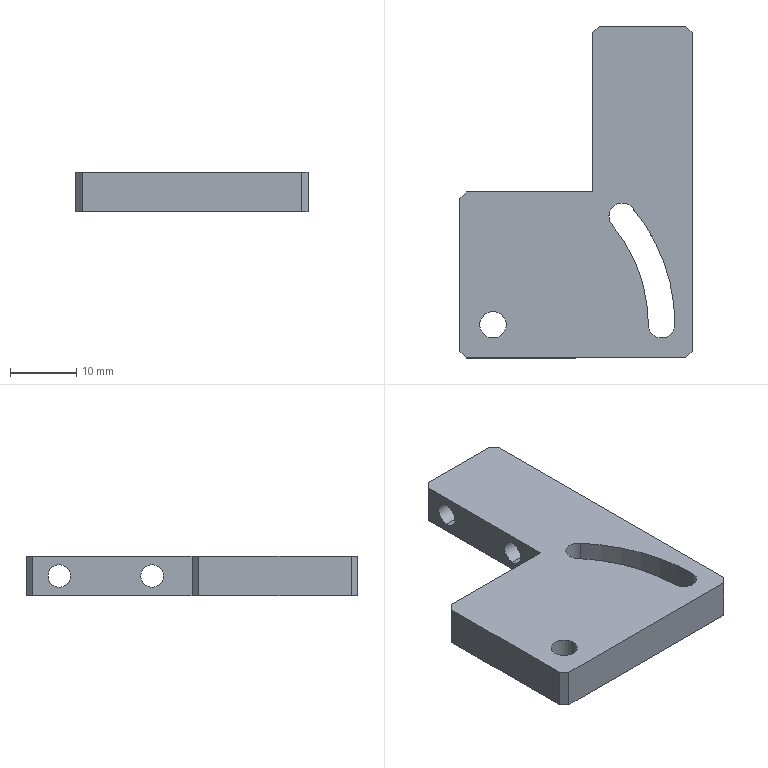Part | SolidWorks | features Chamfer 1, Cut 1, Extrusion 1, HoleWzd 1, ICE 1 | 1 solid | 23 faces | box 35 x 50 x 6 mm | volume 6636 mm3 | plane 13 | cylinder 10 | commonest cylinder face diameters 3.4 x4 4 x4 46.8 x1 54.8 x1
STEP:
#1=CARTESIAN_POINT('',(17.5,20.,-1.7));
#2=VERTEX_POINT('',#1);
#3=CARTESIAN_POINT('',(17.5,20.,1.7));
#4=VERTEX_POINT('',#3);
#5=CARTESIAN_POINT('',(17.5,20.,0.));
#6=DIRECTION('',(-1.,0.,0.));
#7=DIRECTION('',(0.,0.,1.));
#8=AXIS2_PLACEMENT_3D('',#5,#6,#7);
#9=CIRCLE('',#8,1.7);
#10=EDGE_CURVE('',#2,#4,#9,.T.);
#11=ORIENTED_EDGE('',*,*,#10,.F.);
#12=CARTESIAN_POINT('',(2.5,20.,-1.7));
#13=VERTEX_POINT('',#12);
#14=CARTESIAN_POINT('',(2.5,20.,-1.7));
#15=DIRECTION('',(-1.,0.,0.));
#16=VECTOR('',#15,1000.);
#17=LINE('',#14,#16);
#18=EDGE_CURVE('',#2,#13,#17,.T.);
#19=ORIENTED_EDGE('',*,*,#18,.T.);
#20=CARTESIAN_POINT('',(2.5,20.,1.7));
#21=VERTEX_POINT('',#20);
#22=CARTESIAN_POINT('',(2.5,20.,0.));
#23=DIRECTION('',(-1.,0.,0.));
#24=DIRECTION('',(0.,0.,1.));
#25=AXIS2_PLACEMENT_3D('',#22,#23,#24);
#26=CIRCLE('',#25,1.7);
#27=EDGE_CURVE('',#13,#21,#26,.T.);
#28=ORIENTED_EDGE('',*,*,#27,.T.);
#29=CARTESIAN_POINT('',(2.5,20.,1.7));
#30=DIRECTION('',(-1.,0.,0.));
#31=VECTOR('',#30,1000.);
#32=LINE('',#29,#31);
#33=EDGE_CURVE('',#4,#21,#32,.T.);
#34=ORIENTED_EDGE('',*,*,#33,.F.);
#35=EDGE_LOOP('',(#11,#19,#28,#34));
#36=FACE_OUTER_BOUND('',#35,.T.);
#37=CARTESIAN_POINT('',(2.5,20.,0.));
#38=DIRECTION('',(-1.,0.,0.));
#39=DIRECTION('',(0.,0.,1.));
#40=AXIS2_PLACEMENT_3D('',#37,#38,#39);
#41=CYLINDRICAL_SURFACE('',#40,1.7);
#42=ADVANCED_FACE('',(#36),#41,.F.);
#43=CARTESIAN_POINT('',(17.5,6.,-1.7));
#44=VERTEX_POINT('',#43);
#45=CARTESIAN_POINT('',(17.5,6.,1.7));
#46=VERTEX_POINT('',#45);
#47=CARTESIAN_POINT('',(17.5,6.,0.));
#48=DIRECTION('',(-1.,0.,0.));
#49=DIRECTION('',(0.,0.,1.));
#50=AXIS2_PLACEMENT_3D('',#47,#48,#49);
#51=CIRCLE('',#50,1.7);
#52=EDGE_CURVE('',#44,#46,#51,.T.);
#53=ORIENTED_EDGE('',*,*,#52,.F.);
#54=CARTESIAN_POINT('',(2.5,6.,-1.7));
#55=VERTEX_POINT('',#54);
#56=CARTESIAN_POINT('',(2.5,6.,-1.7));
#57=DIRECTION('',(-1.,0.,0.));
#58=VECTOR('',#57,1000.);
#59=LINE('',#56,#58);
#60=EDGE_CURVE('',#44,#55,#59,.T.);
#61=ORIENTED_EDGE('',*,*,#60,.T.);
#62=CARTESIAN_POINT('',(2.5,6.,1.7));
#63=VERTEX_POINT('',#62);
#64=CARTESIAN_POINT('',(2.5,6.,0.));
#65=DIRECTION('',(-1.,0.,0.));
#66=DIRECTION('',(0.,0.,1.));
#67=AXIS2_PLACEMENT_3D('',#64,#65,#66);
#68=CIRCLE('',#67,1.7);
#69=EDGE_CURVE('',#55,#63,#68,.T.);
#70=ORIENTED_EDGE('',*,*,#69,.T.);
#71=CARTESIAN_POINT('',(2.5,6.,1.7));
#72=DIRECTION('',(-1.,0.,0.));
#73=VECTOR('',#72,1000.);
#74=LINE('',#71,#73);
#75=EDGE_CURVE('',#46,#63,#74,.T.);
#76=ORIENTED_EDGE('',*,*,#75,.F.);
#77=EDGE_LOOP('',(#53,#61,#70,#76));
#78=FACE_OUTER_BOUND('',#77,.T.);
#79=CARTESIAN_POINT('',(2.5,6.,0.));
#80=DIRECTION('',(-1.,0.,0.));
#81=DIRECTION('',(0.,0.,1.));
#82=AXIS2_PLACEMENT_3D('',#79,#80,#81);
#83=CYLINDRICAL_SURFACE('',#82,1.7);
#84=ADVANCED_FACE('',(#78),#83,.F.);
#85=CARTESIAN_POINT('',(-14.5,-20.,-3.));
#86=VERTEX_POINT('',#85);
#87=CARTESIAN_POINT('',(-10.5,-20.,-3.));
#88=VERTEX_POINT('',#87);
#89=CARTESIAN_POINT('',(-12.5,-20.,-3.));
#90=DIRECTION('',(0.,0.,1.));
#91=DIRECTION('',(1.,0.,0.));
#92=AXIS2_PLACEMENT_3D('',#89,#90,#91);
#93=CIRCLE('',#92,2.);
#94=EDGE_CURVE('',#86,#88,#93,.T.);
#95=ORIENTED_EDGE('',*,*,#94,.F.);
#96=CARTESIAN_POINT('',(-14.5,-20.,3.));
#97=VERTEX_POINT('',#96);
#98=CARTESIAN_POINT('',(-14.5,-20.,-3.));
#99=DIRECTION('',(0.,0.,1.));
#100=VECTOR('',#99,1000.);
#101=LINE('',#98,#100);
#102=EDGE_CURVE('',#86,#97,#101,.T.);
#103=ORIENTED_EDGE('',*,*,#102,.T.);
#104=CARTESIAN_POINT('',(-10.5,-20.,3.));
#105=VERTEX_POINT('',#104);
#106=CARTESIAN_POINT('',(-12.5,-20.,3.));
#107=DIRECTION('',(0.,0.,1.));
#108=DIRECTION('',(1.,0.,0.));
#109=AXIS2_PLACEMENT_3D('',#106,#107,#108);
#110=CIRCLE('',#109,2.);
#111=EDGE_CURVE('',#97,#105,#110,.T.);
#112=ORIENTED_EDGE('',*,*,#111,.T.);
#113=CARTESIAN_POINT('',(-10.5,-20.,-3.));
#114=DIRECTION('',(0.,0.,1.));
#115=VECTOR('',#114,1000.);
#116=LINE('',#113,#115);
#117=EDGE_CURVE('',#88,#105,#116,.T.);
#118=ORIENTED_EDGE('',*,*,#117,.F.);
#119=EDGE_LOOP('',(#95,#103,#112,#118));
#120=FACE_OUTER_BOUND('',#119,.T.);
#121=CARTESIAN_POINT('',(-12.5,-20.,-3.));
#122=DIRECTION('',(0.,0.,1.));
#123=DIRECTION('',(1.,0.,0.));
#124=AXIS2_PLACEMENT_3D('',#121,#122,#123);
#125=CYLINDRICAL_SURFACE('',#124,2.);
#126=ADVANCED_FACE('',(#120),#125,.F.);
#127=CARTESIAN_POINT('',(-17.5,-1.,-3.));
#128=VERTEX_POINT('',#127);
#129=CARTESIAN_POINT('',(-17.5,-24.,-3.));
#130=VERTEX_POINT('',#129);
#131=CARTESIAN_POINT('',(-17.5,-25.,-3.));
#132=DIRECTION('',(0.,-1.,0.));
#133=VECTOR('',#132,1000.);
#134=LINE('',#131,#133);
#135=EDGE_CURVE('',#128,#130,#134,.T.);
#136=ORIENTED_EDGE('',*,*,#135,.T.);
#137=CARTESIAN_POINT('',(-17.5,-24.,3.));
#138=VERTEX_POINT('',#137);
#139=CARTESIAN_POINT('',(-17.5,-24.,3.));
#140=DIRECTION('',(0.,0.,1.));
#141=VECTOR('',#140,1000.);
#142=LINE('',#139,#141);
#143=EDGE_CURVE('',#130,#138,#142,.T.);
#144=ORIENTED_EDGE('',*,*,#143,.T.);
#145=CARTESIAN_POINT('',(-17.5,-1.,3.));
#146=VERTEX_POINT('',#145);
#147=CARTESIAN_POINT('',(-17.5,-25.,3.));
#148=DIRECTION('',(0.,-1.,0.));
#149=VECTOR('',#148,1000.);
#150=LINE('',#147,#149);
#151=EDGE_CURVE('',#146,#138,#150,.T.);
#152=ORIENTED_EDGE('',*,*,#151,.F.);
#153=CARTESIAN_POINT('',(-17.5,-1.,3.));
#154=DIRECTION('',(0.,0.,-1.));
#155=VECTOR('',#154,1000.);
#156=LINE('',#153,#155);
#157=EDGE_CURVE('',#146,#128,#156,.T.);
#158=ORIENTED_EDGE('',*,*,#157,.T.);
#159=EDGE_LOOP('',(#136,#144,#152,#158));
#160=FACE_OUTER_BOUND('',#159,.T.);
#161=CARTESIAN_POINT('',(-17.5,-25.,3.));
#162=DIRECTION('',(1.,0.,0.));
#163=DIRECTION('',(0.,0.,-1.));
#164=AXIS2_PLACEMENT_3D('',#161,#162,#163);
#165=PLANE('',#164);
#166=ADVANCED_FACE('',(#160),#165,.F.);
#167=CARTESIAN_POINT('',(-16.5,-25.,-3.));
#168=VERTEX_POINT('',#167);
#169=CARTESIAN_POINT('',(16.5,-25.,-3.));
#170=VERTEX_POINT('',#169);
#171=CARTESIAN_POINT('',(17.5,-25.,-3.));
#172=DIRECTION('',(1.,0.,0.));
#173=VECTOR('',#172,1000.);
#174=LINE('',#171,#173);
#175=EDGE_CURVE('',#168,#170,#174,.T.);
#176=ORIENTED_EDGE('',*,*,#175,.T.);
#177=CARTESIAN_POINT('',(16.5,-25.,3.));
#178=VERTEX_POINT('',#177);
#179=CARTESIAN_POINT('',(16.5,-25.,3.));
#180=DIRECTION('',(0.,0.,1.));
#181=VECTOR('',#180,1000.);
#182=LINE('',#179,#181);
#183=EDGE_CURVE('',#170,#178,#182,.T.);
#184=ORIENTED_EDGE('',*,*,#183,.T.);
#185=CARTESIAN_POINT('',(-16.5,-25.,3.));
#186=VERTEX_POINT('',#185);
#187=CARTESIAN_POINT('',(17.5,-25.,3.));
#188=DIRECTION('',(1.,0.,0.));
#189=VECTOR('',#188,1000.);
#190=LINE('',#187,#189);
#191=EDGE_CURVE('',#186,#178,#190,.T.);
#192=ORIENTED_EDGE('',*,*,#191,.F.);
#193=CARTESIAN_POINT('',(-16.5,-25.,3.));
#194=DIRECTION('',(0.,0.,-1.));
#195=VECTOR('',#194,1000.);
#196=LINE('',#193,#195);
#197=EDGE_CURVE('',#186,#168,#196,.T.);
#198=ORIENTED_EDGE('',*,*,#197,.T.);
#199=EDGE_LOOP('',(#176,#184,#192,#198));
#200=FACE_OUTER_BOUND('',#199,.T.);
#201=CARTESIAN_POINT('',(17.5,-25.,3.));
#202=DIRECTION('',(0.,1.,0.));
#203=DIRECTION('',(-1.,0.,0.));
#204=AXIS2_PLACEMENT_3D('',#201,#202,#203);
#205=PLANE('',#204);
#206=ADVANCED_FACE('',(#200),#205,.F.);
#207=CARTESIAN_POINT('',(17.5,20.,0.));
#208=DIRECTION('',(-1.,0.,0.));
#209=DIRECTION('',(0.,0.,1.));
#210=AXIS2_PLACEMENT_3D('',#207,#208,#209);
#211=CIRCLE('',#210,1.7);
#212=EDGE_CURVE('',#4,#2,#211,.T.);
#213=ORIENTED_EDGE('',*,*,#212,.T.);
#214=ORIENTED_EDGE('',*,*,#10,.T.);
#215=EDGE_LOOP('',(#213,#214));
#216=FACE_BOUND('',#215,.T.);
#217=CARTESIAN_POINT('',(17.5,6.,0.));
#218=DIRECTION('',(-1.,0.,0.));
#219=DIRECTION('',(0.,0.,1.));
#220=AXIS2_PLACEMENT_3D('',#217,#218,#219);
#221=CIRCLE('',#220,1.7);
#222=EDGE_CURVE('',#46,#44,#221,.T.);
#223=ORIENTED_EDGE('',*,*,#222,.T.);
#224=ORIENTED_EDGE('',*,*,#52,.T.);
#225=EDGE_LOOP('',(#223,#224));
#226=FACE_BOUND('',#225,.T.);
#227=CARTESIAN_POINT('',(17.5,-24.,3.));
#228=VERTEX_POINT('',#227);
#229=CARTESIAN_POINT('',(17.5,24.,3.));
#230=VERTEX_POINT('',#229);
#231=CARTESIAN_POINT('',(17.5,-25.,3.));
#232=DIRECTION('',(0.,1.,0.));
#233=VECTOR('',#232,1000.);
#234=LINE('',#231,#233);
#235=EDGE_CURVE('',#228,#230,#234,.T.);
#236=ORIENTED_EDGE('',*,*,#235,.F.);
#237=CARTESIAN_POINT('',(17.5,-24.,-3.));
#238=VERTEX_POINT('',#237);
#239=CARTESIAN_POINT('',(17.5,-24.,3.));
#240=DIRECTION('',(0.,0.,-1.));
#241=VECTOR('',#240,1000.);
#242=LINE('',#239,#241);
#243=EDGE_CURVE('',#228,#238,#242,.T.);
#244=ORIENTED_EDGE('',*,*,#243,.T.);
#245=CARTESIAN_POINT('',(17.5,24.,-3.));
#246=VERTEX_POINT('',#245);
#247=CARTESIAN_POINT('',(17.5,-25.,-3.));
#248=DIRECTION('',(0.,1.,0.));
#249=VECTOR('',#248,1000.);
#250=LINE('',#247,#249);
#251=EDGE_CURVE('',#238,#246,#250,.T.);
#252=ORIENTED_EDGE('',*,*,#251,.T.);
#253=CARTESIAN_POINT('',(17.5,24.,3.));
#254=DIRECTION('',(0.,0.,1.));
#255=VECTOR('',#254,1000.);
#256=LINE('',#253,#255);
#257=EDGE_CURVE('',#246,#230,#256,.T.);
#258=ORIENTED_EDGE('',*,*,#257,.T.);
#259=EDGE_LOOP('',(#236,#244,#252,#258));
#260=FACE_OUTER_BOUND('',#259,.T.);
#261=CARTESIAN_POINT('',(17.5,-25.,3.));
#262=DIRECTION('',(-1.,0.,0.));
#263=DIRECTION('',(0.,0.,1.));
#264=AXIS2_PLACEMENT_3D('',#261,#262,#263);
#265=PLANE('',#264);
#266=ADVANCED_FACE('',(#216,#226,#260),#265,.F.);
#267=CARTESIAN_POINT('',(16.5,25.,3.));
#268=VERTEX_POINT('',#267);
#269=CARTESIAN_POINT('',(3.5,25.,3.));
#270=VERTEX_POINT('',#269);
#271=CARTESIAN_POINT('',(17.5,25.,3.));
#272=DIRECTION('',(-1.,0.,0.));
#273=VECTOR('',#272,1000.);
#274=LINE('',#271,#273);
#275=EDGE_CURVE('',#268,#270,#274,.T.);
#276=ORIENTED_EDGE('',*,*,#275,.F.);
#277=CARTESIAN_POINT('',(16.5,25.,-3.));
#278=VERTEX_POINT('',#277);
#279=CARTESIAN_POINT('',(16.5,25.,3.));
#280=DIRECTION('',(0.,0.,-1.));
#281=VECTOR('',#280,1000.);
#282=LINE('',#279,#281);
#283=EDGE_CURVE('',#268,#278,#282,.T.);
#284=ORIENTED_EDGE('',*,*,#283,.T.);
#285=CARTESIAN_POINT('',(3.5,25.,-3.));
#286=VERTEX_POINT('',#285);
#287=CARTESIAN_POINT('',(17.5,25.,-3.));
#288=DIRECTION('',(-1.,0.,0.));
#289=VECTOR('',#288,1000.);
#290=LINE('',#287,#289);
#291=EDGE_CURVE('',#278,#286,#290,.T.);
#292=ORIENTED_EDGE('',*,*,#291,.T.);
#293=CARTESIAN_POINT('',(3.5,25.,3.));
#294=DIRECTION('',(0.,0.,1.));
#295=VECTOR('',#294,1000.);
#296=LINE('',#293,#295);
#297=EDGE_CURVE('',#286,#270,#296,.T.);
#298=ORIENTED_EDGE('',*,*,#297,.T.);
#299=EDGE_LOOP('',(#276,#284,#292,#298));
#300=FACE_OUTER_BOUND('',#299,.T.);
#301=CARTESIAN_POINT('',(17.5,25.,3.));
#302=DIRECTION('',(0.,-1.,0.));
#303=DIRECTION('',(1.,0.,0.));
#304=AXIS2_PLACEMENT_3D('',#301,#302,#303);
#305=PLANE('',#304);
#306=ADVANCED_FACE('',(#300),#305,.F.);
#307=CARTESIAN_POINT('',(-12.5,-20.,3.));
#308=DIRECTION('',(0.,0.,1.));
#309=DIRECTION('',(1.,0.,0.));
#310=AXIS2_PLACEMENT_3D('',#307,#308,#309);
#311=CIRCLE('',#310,2.);
#312=EDGE_CURVE('',#105,#97,#311,.T.);
#313=ORIENTED_EDGE('',*,*,#312,.F.);
#314=ORIENTED_EDGE('',*,*,#111,.F.);
#315=EDGE_LOOP('',(#313,#314));
#316=FACE_BOUND('',#315,.T.);
#317=CARTESIAN_POINT('',(10.9,-20.,3.));
#318=VERTEX_POINT('',#317);
#319=CARTESIAN_POINT('',(14.9,-20.,3.));
#320=VERTEX_POINT('',#319);
#321=CARTESIAN_POINT('',(12.9,-20.,3.));
#322=DIRECTION('',(0.,0.,1.));
#323=DIRECTION('',(1.,0.,0.));
#324=AXIS2_PLACEMENT_3D('',#321,#322,#323);
#325=CIRCLE('',#324,2.);
#326=EDGE_CURVE('',#318,#320,#325,.T.);
#327=ORIENTED_EDGE('',*,*,#326,.F.);
#328=CARTESIAN_POINT('',(5.425,-4.959,3.));
#329=VERTEX_POINT('',#328);
#330=CARTESIAN_POINT('',(-12.5,-20.,3.));
#331=DIRECTION('',(0.,0.,-1.));
#332=DIRECTION('',(1.,0.,0.));
#333=AXIS2_PLACEMENT_3D('',#330,#331,#332);
#334=CIRCLE('',#333,23.4);
#335=EDGE_CURVE('',#329,#318,#334,.T.);
#336=ORIENTED_EDGE('',*,*,#335,.F.);
#337=CARTESIAN_POINT('',(8.49,-2.388,3.));
#338=VERTEX_POINT('',#337);
#339=CARTESIAN_POINT('',(6.958,-3.673,3.));
#340=DIRECTION('',(0.,0.,1.));
#341=DIRECTION('',(1.,0.,0.));
#342=AXIS2_PLACEMENT_3D('',#339,#340,#341);
#343=CIRCLE('',#342,2.);
#344=EDGE_CURVE('',#338,#329,#343,.T.);
#345=ORIENTED_EDGE('',*,*,#344,.F.);
#346=CARTESIAN_POINT('',(-12.5,-20.,3.));
#347=DIRECTION('',(0.,0.,1.));
#348=DIRECTION('',(1.,0.,0.));
#349=AXIS2_PLACEMENT_3D('',#346,#347,#348);
#350=CIRCLE('',#349,27.4);
#351=EDGE_CURVE('',#320,#338,#350,.T.);
#352=ORIENTED_EDGE('',*,*,#351,.F.);
#353=EDGE_LOOP('',(#327,#336,#345,#352));
#354=FACE_BOUND('',#353,.T.);
#355=ORIENTED_EDGE('',*,*,#191,.T.);
#356=CARTESIAN_POINT('',(20.75,-20.75,3.));
#357=DIRECTION('',(0.7071,0.7071,0.));
#358=VECTOR('',#357,1000.);
#359=LINE('',#356,#358);
#360=EDGE_CURVE('',#178,#228,#359,.T.);
#361=ORIENTED_EDGE('',*,*,#360,.T.);
#362=ORIENTED_EDGE('',*,*,#235,.T.);
#363=CARTESIAN_POINT('',(20.75,20.75,3.));
#364=DIRECTION('',(-0.7071,0.7071,0.));
#365=VECTOR('',#364,1000.);
#366=LINE('',#363,#365);
#367=EDGE_CURVE('',#230,#268,#366,.T.);
#368=ORIENTED_EDGE('',*,*,#367,.T.);
#369=ORIENTED_EDGE('',*,*,#275,.T.);
#370=CARTESIAN_POINT('',(2.5,24.,3.));
#371=VERTEX_POINT('',#370);
#372=CARTESIAN_POINT('',(-10.75,10.75,3.));
#373=DIRECTION('',(-0.7071,-0.7071,0.));
#374=VECTOR('',#373,1000.);
#375=LINE('',#372,#374);
#376=EDGE_CURVE('',#270,#371,#375,.T.);
#377=ORIENTED_EDGE('',*,*,#376,.T.);
#378=CARTESIAN_POINT('',(2.5,0.,3.));
#379=VERTEX_POINT('',#378);
#380=CARTESIAN_POINT('',(2.5,25.,3.));
#381=DIRECTION('',(0.,1.,0.));
#382=VECTOR('',#381,1000.);
#383=LINE('',#380,#382);
#384=EDGE_CURVE('',#379,#371,#383,.T.);
#385=ORIENTED_EDGE('',*,*,#384,.F.);
#386=CARTESIAN_POINT('',(-16.5,0.,3.));
#387=VERTEX_POINT('',#386);
#388=CARTESIAN_POINT('',(-17.5,0.,3.));
#389=DIRECTION('',(1.,0.,0.));
#390=VECTOR('',#389,1000.);
#391=LINE('',#388,#390);
#392=EDGE_CURVE('',#387,#379,#391,.T.);
#393=ORIENTED_EDGE('',*,*,#392,.F.);
#394=CARTESIAN_POINT('',(-8.25,8.25,3.));
#395=DIRECTION('',(-0.7071,-0.7071,0.));
#396=VECTOR('',#395,1000.);
#397=LINE('',#394,#396);
#398=EDGE_CURVE('',#387,#146,#397,.T.);
#399=ORIENTED_EDGE('',*,*,#398,.T.);
#400=ORIENTED_EDGE('',*,*,#151,.T.);
#401=CARTESIAN_POINT('',(-20.75,-20.75,3.));
#402=DIRECTION('',(0.7071,-0.7071,0.));
#403=VECTOR('',#402,1000.);
#404=LINE('',#401,#403);
#405=EDGE_CURVE('',#138,#186,#404,.T.);
#406=ORIENTED_EDGE('',*,*,#405,.T.);
#407=EDGE_LOOP('',(#355,#361,#362,#368,#369,#377,#385,#393,#399,#400,#406));
#408=FACE_OUTER_BOUND('',#407,.T.);
#409=CARTESIAN_POINT('',(0.,0.,3.));
#410=DIRECTION('',(0.,0.,1.));
#411=DIRECTION('',(1.,0.,0.));
#412=AXIS2_PLACEMENT_3D('',#409,#410,#411);
#413=PLANE('',#412);
#414=ADVANCED_FACE('',(#316,#354,#408),#413,.T.);
#415=CARTESIAN_POINT('',(-12.5,-20.,-3.));
#416=DIRECTION('',(0.,0.,1.));
#417=DIRECTION('',(1.,0.,0.));
#418=AXIS2_PLACEMENT_3D('',#415,#416,#417);
#419=CIRCLE('',#418,2.);
#420=EDGE_CURVE('',#88,#86,#419,.T.);
#421=ORIENTED_EDGE('',*,*,#420,.T.);
#422=ORIENTED_EDGE('',*,*,#94,.T.);
#423=EDGE_LOOP('',(#421,#422));
#424=FACE_BOUND('',#423,.T.);
#425=CARTESIAN_POINT('',(5.425,-4.959,-3.));
#426=VERTEX_POINT('',#425);
#427=CARTESIAN_POINT('',(10.9,-20.,-3.));
#428=VERTEX_POINT('',#427);
#429=CARTESIAN_POINT('',(-12.5,-20.,-3.));
#430=DIRECTION('',(0.,0.,-1.));
#431=DIRECTION('',(1.,0.,0.));
#432=AXIS2_PLACEMENT_3D('',#429,#430,#431);
#433=CIRCLE('',#432,23.4);
#434=EDGE_CURVE('',#426,#428,#433,.T.);
#435=ORIENTED_EDGE('',*,*,#434,.T.);
#436=CARTESIAN_POINT('',(14.9,-20.,-3.));
#437=VERTEX_POINT('',#436);
#438=CARTESIAN_POINT('',(12.9,-20.,-3.));
#439=DIRECTION('',(0.,0.,1.));
#440=DIRECTION('',(1.,0.,0.));
#441=AXIS2_PLACEMENT_3D('',#438,#439,#440);
#442=CIRCLE('',#441,2.);
#443=EDGE_CURVE('',#428,#437,#442,.T.);
#444=ORIENTED_EDGE('',*,*,#443,.T.);
#445=CARTESIAN_POINT('',(8.49,-2.388,-3.));
#446=VERTEX_POINT('',#445);
#447=CARTESIAN_POINT('',(-12.5,-20.,-3.));
#448=DIRECTION('',(0.,0.,1.));
#449=DIRECTION('',(1.,0.,0.));
#450=AXIS2_PLACEMENT_3D('',#447,#448,#449);
#451=CIRCLE('',#450,27.4);
#452=EDGE_CURVE('',#437,#446,#451,.T.);
#453=ORIENTED_EDGE('',*,*,#452,.T.);
#454=CARTESIAN_POINT('',(6.958,-3.673,-3.));
#455=DIRECTION('',(0.,0.,1.));
#456=DIRECTION('',(1.,0.,0.));
#457=AXIS2_PLACEMENT_3D('',#454,#455,#456);
#458=CIRCLE('',#457,2.);
#459=EDGE_CURVE('',#446,#426,#458,.T.);
#460=ORIENTED_EDGE('',*,*,#459,.T.);
#461=EDGE_LOOP('',(#435,#444,#453,#460));
#462=FACE_BOUND('',#461,.T.);
#463=ORIENTED_EDGE('',*,*,#251,.F.);
#464=CARTESIAN_POINT('',(17.5,-24.,-3.));
#465=DIRECTION('',(-0.7071,-0.7071,0.));
#466=VECTOR('',#465,1000.);
#467=LINE('',#464,#466);
#468=EDGE_CURVE('',#238,#170,#467,.T.);
#469=ORIENTED_EDGE('',*,*,#468,.T.);
#470=ORIENTED_EDGE('',*,*,#175,.F.);
#471=CARTESIAN_POINT('',(-16.5,-25.,-3.));
#472=DIRECTION('',(-0.7071,0.7071,0.));
#473=VECTOR('',#472,1000.);
#474=LINE('',#471,#473);
#475=EDGE_CURVE('',#168,#130,#474,.T.);
#476=ORIENTED_EDGE('',*,*,#475,.T.);
#477=ORIENTED_EDGE('',*,*,#135,.F.);
#478=CARTESIAN_POINT('',(-16.5,0.,-3.));
#479=VERTEX_POINT('',#478);
#480=CARTESIAN_POINT('',(-16.5,0.,-3.));
#481=DIRECTION('',(0.7071,0.7071,0.));
#482=VECTOR('',#481,1000.);
#483=LINE('',#480,#482);
#484=EDGE_CURVE('',#128,#479,#483,.T.);
#485=ORIENTED_EDGE('',*,*,#484,.T.);
#486=CARTESIAN_POINT('',(2.5,0.,-3.));
#487=VERTEX_POINT('',#486);
#488=CARTESIAN_POINT('',(-17.5,0.,-3.));
#489=DIRECTION('',(1.,0.,0.));
#490=VECTOR('',#489,1000.);
#491=LINE('',#488,#490);
#492=EDGE_CURVE('',#479,#487,#491,.T.);
#493=ORIENTED_EDGE('',*,*,#492,.T.);
#494=CARTESIAN_POINT('',(2.5,24.,-3.));
#495=VERTEX_POINT('',#494);
#496=CARTESIAN_POINT('',(2.5,25.,-3.));
#497=DIRECTION('',(0.,1.,0.));
#498=VECTOR('',#497,1000.);
#499=LINE('',#496,#498);
#500=EDGE_CURVE('',#487,#495,#499,.T.);
#501=ORIENTED_EDGE('',*,*,#500,.T.);
#502=CARTESIAN_POINT('',(3.5,25.,-3.));
#503=DIRECTION('',(0.7071,0.7071,0.));
#504=VECTOR('',#503,1000.);
#505=LINE('',#502,#504);
#506=EDGE_CURVE('',#495,#286,#505,.T.);
#507=ORIENTED_EDGE('',*,*,#506,.T.);
#508=ORIENTED_EDGE('',*,*,#291,.F.);
#509=CARTESIAN_POINT('',(16.5,25.,-3.));
#510=DIRECTION('',(0.7071,-0.7071,0.));
#511=VECTOR('',#510,1000.);
#512=LINE('',#509,#511);
#513=EDGE_CURVE('',#278,#246,#512,.T.);
#514=ORIENTED_EDGE('',*,*,#513,.T.);
#515=EDGE_LOOP('',(#463,#469,#470,#476,#477,#485,#493,#501,#507,#508,#514));
#516=FACE_OUTER_BOUND('',#515,.T.);
#517=CARTESIAN_POINT('',(0.,0.,-3.));
#518=DIRECTION('',(0.,0.,1.));
#519=DIRECTION('',(1.,0.,0.));
#520=AXIS2_PLACEMENT_3D('',#517,#518,#519);
#521=PLANE('',#520);
#522=ADVANCED_FACE('',(#424,#462,#516),#521,.F.);
#523=CARTESIAN_POINT('',(2.5,20.,0.));
#524=DIRECTION('',(-1.,0.,0.));
#525=DIRECTION('',(0.,0.,1.));
#526=AXIS2_PLACEMENT_3D('',#523,#524,#525);
#527=CIRCLE('',#526,1.7);
#528=EDGE_CURVE('',#21,#13,#527,.T.);
#529=ORIENTED_EDGE('',*,*,#528,.F.);
#530=ORIENTED_EDGE('',*,*,#27,.F.);
#531=EDGE_LOOP('',(#529,#530));
#532=FACE_BOUND('',#531,.T.);
#533=CARTESIAN_POINT('',(2.5,6.,0.));
#534=DIRECTION('',(-1.,0.,0.));
#535=DIRECTION('',(0.,0.,1.));
#536=AXIS2_PLACEMENT_3D('',#533,#534,#535);
#537=CIRCLE('',#536,1.7);
#538=EDGE_CURVE('',#63,#55,#537,.T.);
#539=ORIENTED_EDGE('',*,*,#538,.F.);
#540=ORIENTED_EDGE('',*,*,#69,.F.);
#541=EDGE_LOOP('',(#539,#540));
#542=FACE_BOUND('',#541,.T.);
#543=ORIENTED_EDGE('',*,*,#384,.T.);
#544=CARTESIAN_POINT('',(2.5,24.,-3.));
#545=DIRECTION('',(0.,0.,-1.));
#546=VECTOR('',#545,1000.);
#547=LINE('',#544,#546);
#548=EDGE_CURVE('',#371,#495,#547,.T.);
#549=ORIENTED_EDGE('',*,*,#548,.T.);
#550=ORIENTED_EDGE('',*,*,#500,.F.);
#551=CARTESIAN_POINT('',(2.5,0.,-3.));
#552=DIRECTION('',(0.,0.,1.));
#553=VECTOR('',#552,1000.);
#554=LINE('',#551,#553);
#555=EDGE_CURVE('',#487,#379,#554,.T.);
#556=ORIENTED_EDGE('',*,*,#555,.T.);
#557=EDGE_LOOP('',(#543,#549,#550,#556));
#558=FACE_OUTER_BOUND('',#557,.T.);
#559=CARTESIAN_POINT('',(2.5,25.,-3.));
#560=DIRECTION('',(1.,0.,0.));
#561=DIRECTION('',(0.,1.,0.));
#562=AXIS2_PLACEMENT_3D('',#559,#560,#561);
#563=PLANE('',#562);
#564=ADVANCED_FACE('',(#532,#542,#558),#563,.F.);
#565=ORIENTED_EDGE('',*,*,#492,.F.);
#566=CARTESIAN_POINT('',(-16.5,0.,-3.));
#567=DIRECTION('',(0.,0.,1.));
#568=VECTOR('',#567,1000.);
#569=LINE('',#566,#568);
#570=EDGE_CURVE('',#479,#387,#569,.T.);
#571=ORIENTED_EDGE('',*,*,#570,.T.);
#572=ORIENTED_EDGE('',*,*,#392,.T.);
#573=ORIENTED_EDGE('',*,*,#555,.F.);
#574=EDGE_LOOP('',(#565,#571,#572,#573));
#575=FACE_OUTER_BOUND('',#574,.T.);
#576=CARTESIAN_POINT('',(-17.5,0.,-3.));
#577=DIRECTION('',(0.,-1.,0.));
#578=DIRECTION('',(1.,0.,0.));
#579=AXIS2_PLACEMENT_3D('',#576,#577,#578);
#580=PLANE('',#579);
#581=ADVANCED_FACE('',(#575),#580,.F.);
#582=ORIENTED_EDGE('',*,*,#326,.T.);
#583=CARTESIAN_POINT('',(14.9,-20.,-3.));
#584=DIRECTION('',(0.,0.,1.));
#585=VECTOR('',#584,1000.);
#586=LINE('',#583,#585);
#587=EDGE_CURVE('',#437,#320,#586,.T.);
#588=ORIENTED_EDGE('',*,*,#587,.F.);
#589=ORIENTED_EDGE('',*,*,#443,.F.);
#590=CARTESIAN_POINT('',(10.9,-20.,-3.));
#591=DIRECTION('',(0.,0.,1.));
#592=VECTOR('',#591,1000.);
#593=LINE('',#590,#592);
#594=EDGE_CURVE('',#428,#318,#593,.T.);
#595=ORIENTED_EDGE('',*,*,#594,.T.);
#596=EDGE_LOOP('',(#582,#588,#589,#595));
#597=FACE_OUTER_BOUND('',#596,.T.);
#598=CARTESIAN_POINT('',(12.9,-20.,-3.));
#599=DIRECTION('',(0.,0.,1.));
#600=DIRECTION('',(1.,0.,0.));
#601=AXIS2_PLACEMENT_3D('',#598,#599,#600);
#602=CYLINDRICAL_SURFACE('',#601,2.);
#603=ADVANCED_FACE('',(#597),#602,.F.);
#604=ORIENTED_EDGE('',*,*,#335,.T.);
#605=ORIENTED_EDGE('',*,*,#594,.F.);
#606=ORIENTED_EDGE('',*,*,#434,.F.);
#607=CARTESIAN_POINT('',(5.425,-4.959,-3.));
#608=DIRECTION('',(0.,0.,1.));
#609=VECTOR('',#608,1000.);
#610=LINE('',#607,#609);
#611=EDGE_CURVE('',#426,#329,#610,.T.);
#612=ORIENTED_EDGE('',*,*,#611,.T.);
#613=EDGE_LOOP('',(#604,#605,#606,#612));
#614=FACE_OUTER_BOUND('',#613,.T.);
#615=CARTESIAN_POINT('',(-12.5,-20.,-3.));
#616=DIRECTION('',(0.,0.,1.));
#617=DIRECTION('',(1.,0.,0.));
#618=AXIS2_PLACEMENT_3D('',#615,#616,#617);
#619=CYLINDRICAL_SURFACE('',#618,23.4);
#620=ADVANCED_FACE('',(#614),#619,.T.);
#621=ORIENTED_EDGE('',*,*,#344,.T.);
#622=ORIENTED_EDGE('',*,*,#611,.F.);
#623=ORIENTED_EDGE('',*,*,#459,.F.);
#624=CARTESIAN_POINT('',(8.49,-2.388,-3.));
#625=DIRECTION('',(0.,0.,1.));
#626=VECTOR('',#625,1000.);
#627=LINE('',#624,#626);
#628=EDGE_CURVE('',#446,#338,#627,.T.);
#629=ORIENTED_EDGE('',*,*,#628,.T.);
#630=EDGE_LOOP('',(#621,#622,#623,#629));
#631=FACE_OUTER_BOUND('',#630,.T.);
#632=CARTESIAN_POINT('',(6.958,-3.673,-3.));
#633=DIRECTION('',(0.,0.,1.));
#634=DIRECTION('',(1.,0.,0.));
#635=AXIS2_PLACEMENT_3D('',#632,#633,#634);
#636=CYLINDRICAL_SURFACE('',#635,2.);
#637=ADVANCED_FACE('',(#631),#636,.F.);
#638=ORIENTED_EDGE('',*,*,#351,.T.);
#639=ORIENTED_EDGE('',*,*,#628,.F.);
#640=ORIENTED_EDGE('',*,*,#452,.F.);
#641=ORIENTED_EDGE('',*,*,#587,.T.);
#642=EDGE_LOOP('',(#638,#639,#640,#641));
#643=FACE_OUTER_BOUND('',#642,.T.);
#644=CARTESIAN_POINT('',(-12.5,-20.,-3.));
#645=DIRECTION('',(0.,0.,1.));
#646=DIRECTION('',(1.,0.,0.));
#647=AXIS2_PLACEMENT_3D('',#644,#645,#646);
#648=CYLINDRICAL_SURFACE('',#647,27.4);
#649=ADVANCED_FACE('',(#643),#648,.F.);
#650=ORIENTED_EDGE('',*,*,#102,.F.);
#651=ORIENTED_EDGE('',*,*,#420,.F.);
#652=ORIENTED_EDGE('',*,*,#117,.T.);
#653=ORIENTED_EDGE('',*,*,#312,.T.);
#654=EDGE_LOOP('',(#650,#651,#652,#653));
#655=FACE_OUTER_BOUND('',#654,.T.);
#656=CARTESIAN_POINT('',(-12.5,-20.,-3.));
#657=DIRECTION('',(0.,0.,1.));
#658=DIRECTION('',(1.,0.,0.));
#659=AXIS2_PLACEMENT_3D('',#656,#657,#658);
#660=CYLINDRICAL_SURFACE('',#659,2.);
#661=ADVANCED_FACE('',(#655),#660,.F.);
#662=ORIENTED_EDGE('',*,*,#60,.F.);
#663=ORIENTED_EDGE('',*,*,#222,.F.);
#664=ORIENTED_EDGE('',*,*,#75,.T.);
#665=ORIENTED_EDGE('',*,*,#538,.T.);
#666=EDGE_LOOP('',(#662,#663,#664,#665));
#667=FACE_OUTER_BOUND('',#666,.T.);
#668=CARTESIAN_POINT('',(2.5,6.,0.));
#669=DIRECTION('',(-1.,0.,0.));
#670=DIRECTION('',(0.,0.,1.));
#671=AXIS2_PLACEMENT_3D('',#668,#669,#670);
#672=CYLINDRICAL_SURFACE('',#671,1.7);
#673=ADVANCED_FACE('',(#667),#672,.F.);
#674=ORIENTED_EDGE('',*,*,#18,.F.);
#675=ORIENTED_EDGE('',*,*,#212,.F.);
#676=ORIENTED_EDGE('',*,*,#33,.T.);
#677=ORIENTED_EDGE('',*,*,#528,.T.);
#678=EDGE_LOOP('',(#674,#675,#676,#677));
#679=FACE_OUTER_BOUND('',#678,.T.);
#680=CARTESIAN_POINT('',(2.5,20.,0.));
#681=DIRECTION('',(-1.,0.,0.));
#682=DIRECTION('',(0.,0.,1.));
#683=AXIS2_PLACEMENT_3D('',#680,#681,#682);
#684=CYLINDRICAL_SURFACE('',#683,1.7);
#685=ADVANCED_FACE('',(#679),#684,.F.);
#686=ORIENTED_EDGE('',*,*,#360,.F.);
#687=ORIENTED_EDGE('',*,*,#183,.F.);
#688=ORIENTED_EDGE('',*,*,#468,.F.);
#689=ORIENTED_EDGE('',*,*,#243,.F.);
#690=EDGE_LOOP('',(#686,#687,#688,#689));
#691=FACE_OUTER_BOUND('',#690,.T.);
#692=CARTESIAN_POINT('',(17.5,-24.,3.));
#693=DIRECTION('',(-0.7071,0.7071,0.));
#694=DIRECTION('',(0.,0.,-1.));
#695=AXIS2_PLACEMENT_3D('',#692,#693,#694);
#696=PLANE('',#695);
#697=ADVANCED_FACE('',(#691),#696,.F.);
#698=ORIENTED_EDGE('',*,*,#367,.F.);
#699=ORIENTED_EDGE('',*,*,#257,.F.);
#700=ORIENTED_EDGE('',*,*,#513,.F.);
#701=ORIENTED_EDGE('',*,*,#283,.F.);
#702=EDGE_LOOP('',(#698,#699,#700,#701));
#703=FACE_OUTER_BOUND('',#702,.T.);
#704=CARTESIAN_POINT('',(16.5,25.,3.));
#705=DIRECTION('',(-0.7071,-0.7071,0.));
#706=DIRECTION('',(0.,0.,-1.));
#707=AXIS2_PLACEMENT_3D('',#704,#705,#706);
#708=PLANE('',#707);
#709=ADVANCED_FACE('',(#703),#708,.F.);
#710=ORIENTED_EDGE('',*,*,#506,.F.);
#711=ORIENTED_EDGE('',*,*,#548,.F.);
#712=ORIENTED_EDGE('',*,*,#376,.F.);
#713=ORIENTED_EDGE('',*,*,#297,.F.);
#714=EDGE_LOOP('',(#710,#711,#712,#713));
#715=FACE_OUTER_BOUND('',#714,.T.);
#716=CARTESIAN_POINT('',(3.5,25.,3.));
#717=DIRECTION('',(0.7071,-0.7071,0.));
#718=DIRECTION('',(0.,0.,1.));
#719=AXIS2_PLACEMENT_3D('',#716,#717,#718);
#720=PLANE('',#719);
#721=ADVANCED_FACE('',(#715),#720,.F.);
#722=ORIENTED_EDGE('',*,*,#405,.F.);
#723=ORIENTED_EDGE('',*,*,#143,.F.);
#724=ORIENTED_EDGE('',*,*,#475,.F.);
#725=ORIENTED_EDGE('',*,*,#197,.F.);
#726=EDGE_LOOP('',(#722,#723,#724,#725));
#727=FACE_OUTER_BOUND('',#726,.T.);
#728=CARTESIAN_POINT('',(-16.5,-25.,3.));
#729=DIRECTION('',(0.7071,0.7071,0.));
#730=DIRECTION('',(0.,0.,-1.));
#731=AXIS2_PLACEMENT_3D('',#728,#729,#730);
#732=PLANE('',#731);
#733=ADVANCED_FACE('',(#727),#732,.F.);
#734=ORIENTED_EDGE('',*,*,#484,.F.);
#735=ORIENTED_EDGE('',*,*,#157,.F.);
#736=ORIENTED_EDGE('',*,*,#398,.F.);
#737=ORIENTED_EDGE('',*,*,#570,.F.);
#738=EDGE_LOOP('',(#734,#735,#736,#737));
#739=FACE_OUTER_BOUND('',#738,.T.);
#740=CARTESIAN_POINT('',(-16.5,0.,-3.));
#741=DIRECTION('',(0.7071,-0.7071,0.));
#742=DIRECTION('',(0.,0.,1.));
#743=AXIS2_PLACEMENT_3D('',#740,#741,#742);
#744=PLANE('',#743);
#745=ADVANCED_FACE('',(#739),#744,.F.);
#746=CLOSED_SHELL('',(#42,#84,#126,#166,#206,#266,#306,#414,#522,#564,#581,#603,#620,#637,#649,#661,#673,#685,#697,#709,#721,#733,#745));
#747=MANIFOLD_SOLID_BREP('',#746);
#748=CARTESIAN_POINT('',(0.,0.,0.));
#749=DIRECTION('',(0.,0.,1.));
#750=DIRECTION('',(1.,0.,0.));
#751=AXIS2_PLACEMENT_3D('',#748,#749,#750);
#752=(LENGTH_UNIT()NAMED_UNIT(*)SI_UNIT(.MILLI.,.METRE.));
#753=UNCERTAINTY_MEASURE_WITH_UNIT(LENGTH_MEASURE(0.00001),#752,'','');
#754=(NAMED_UNIT(*)PLANE_ANGLE_UNIT()SI_UNIT($,.RADIAN.));
#755=(NAMED_UNIT(*)SI_UNIT($,.STERADIAN.)SOLID_ANGLE_UNIT());
#756=(GEOMETRIC_REPRESENTATION_CONTEXT(3)GLOBAL_UNCERTAINTY_ASSIGNED_CONTEXT((#753))GLOBAL_UNIT_ASSIGNED_CONTEXT((#752,#754,#755))REPRESENTATION_CONTEXT('',''));
#757=ADVANCED_BREP_SHAPE_REPRESENTATION('',(#747,#751),#756);